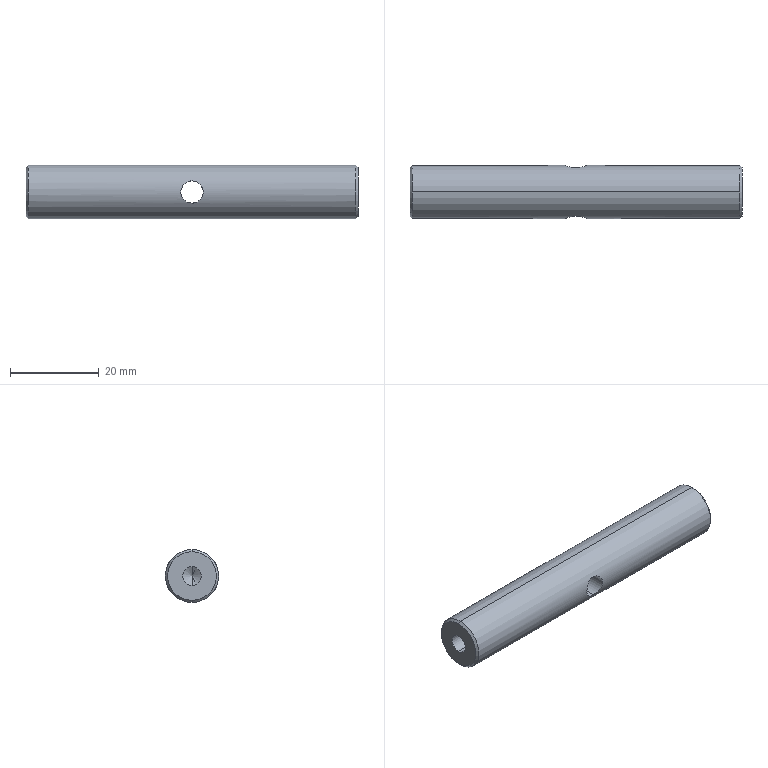Part | SolidWorks | features HoleWzd 2, Chamfer 1, Extrusion 1, ICE 1 | 1 solid | 18 faces | box 75 x 12 x 12 mm | volume 7888 mm3 | cylinder 8 | cone 8 | plane 2 | commonest cylinder face diameters 4.2 x4 5 x2 12 x2
STEP:
#1=CARTESIAN_POINT('',(37.5,-5.454,-2.5));
#2=VERTEX_POINT('',#1);
#3=CARTESIAN_POINT('',(37.5,-5.454,2.5));
#4=VERTEX_POINT('',#3);
#5=CARTESIAN_POINT('',(37.5,-5.454,-2.5));
#6=CARTESIAN_POINT('',(37.335,-5.454,-2.5));
#7=CARTESIAN_POINT('',(37.168,-5.462,-2.483));
#8=CARTESIAN_POINT('',(36.845,-5.491,-2.418));
#9=CARTESIAN_POINT('',(36.688,-5.512,-2.37));
#10=CARTESIAN_POINT('',(36.386,-5.565,-2.244));
#11=CARTESIAN_POINT('',(36.241,-5.596,-2.166));
#12=CARTESIAN_POINT('',(35.972,-5.663,-1.986));
#13=CARTESIAN_POINT('',(35.847,-5.698,-1.882));
#14=CARTESIAN_POINT('',(35.617,-5.769,-1.652));
#15=CARTESIAN_POINT('',(35.515,-5.804,-1.528));
#16=CARTESIAN_POINT('',(35.334,-5.868,-1.259));
#17=CARTESIAN_POINT('',(35.256,-5.898,-1.114));
#18=CARTESIAN_POINT('',(35.13,-5.947,-0.8118));
#19=CARTESIAN_POINT('',(35.082,-5.966,-0.6557));
#20=CARTESIAN_POINT('',(35.017,-5.993,-0.3328));
#21=CARTESIAN_POINT('',(35.,-6.,-0.1652));
#22=CARTESIAN_POINT('',(35.,-6.,0.3293));
#23=CARTESIAN_POINT('',(35.067,-5.971,0.6615));
#24=CARTESIAN_POINT('',(35.256,-5.898,1.114));
#25=CARTESIAN_POINT('',(35.334,-5.868,1.259));
#26=CARTESIAN_POINT('',(35.515,-5.804,1.529));
#27=CARTESIAN_POINT('',(35.618,-5.769,1.653));
#28=CARTESIAN_POINT('',(35.847,-5.698,1.883));
#29=CARTESIAN_POINT('',(35.974,-5.662,1.987));
#30=CARTESIAN_POINT('',(36.242,-5.596,2.166));
#31=CARTESIAN_POINT('',(36.385,-5.565,2.243));
#32=CARTESIAN_POINT('',(36.689,-5.512,2.371));
#33=CARTESIAN_POINT('',(36.845,-5.491,2.418));
#34=CARTESIAN_POINT('',(37.167,-5.462,2.483));
#35=CARTESIAN_POINT('',(37.333,-5.454,2.5));
#36=CARTESIAN_POINT('',(37.5,-5.454,2.5));
#37=B_SPLINE_CURVE_WITH_KNOTS('',3,(#5,#6,#7,#8,#9,#10,#11,#12,#13,#14,#15,#16,#17,#18,#19,#20,#21,#22,#23,#24,#25,#26,#27,#28,#29,#30,#31,#32,#33,#34,#35,#36),.UNSPECIFIED.,.F.,.F.,(4,2,2,2,2,2,2,2,2,2,2,2,2,2,2,4),(0.007907,0.008401,0.008895,0.009388,0.009882,0.01038,0.01087,0.01136,0.01186,0.01284,0.01334,0.01383,0.01433,0.01482,0.01531,0.01581),.UNSPECIFIED.);
#38=EDGE_CURVE('',#2,#4,#37,.T.);
#39=ORIENTED_EDGE('',*,*,#38,.F.);
#40=CARTESIAN_POINT('',(37.5,5.454,-2.5));
#41=VERTEX_POINT('',#40);
#42=CARTESIAN_POINT('',(37.5,-17.,-2.5));
#43=DIRECTION('',(0.,1.,0.));
#44=VECTOR('',#43,1000.);
#45=LINE('',#42,#44);
#46=EDGE_CURVE('',#2,#41,#45,.T.);
#47=ORIENTED_EDGE('',*,*,#46,.T.);
#48=CARTESIAN_POINT('',(37.5,5.454,2.5));
#49=VERTEX_POINT('',#48);
#50=CARTESIAN_POINT('',(37.5,5.454,2.5));
#51=CARTESIAN_POINT('',(37.333,5.454,2.5));
#52=CARTESIAN_POINT('',(37.169,5.462,2.483));
#53=CARTESIAN_POINT('',(36.847,5.491,2.419));
#54=CARTESIAN_POINT('',(36.687,5.513,2.37));
#55=CARTESIAN_POINT('',(36.385,5.565,2.244));
#56=CARTESIAN_POINT('',(36.243,5.596,2.167));
#57=CARTESIAN_POINT('',(35.972,5.663,1.986));
#58=CARTESIAN_POINT('',(35.846,5.699,1.882));
#59=CARTESIAN_POINT('',(35.504,5.804,1.54));
#60=CARTESIAN_POINT('',(35.319,5.873,1.264));
#61=CARTESIAN_POINT('',(35.131,5.947,0.8137));
#62=CARTESIAN_POINT('',(35.081,5.966,0.6541));
#63=CARTESIAN_POINT('',(35.016,5.993,0.3303));
#64=CARTESIAN_POINT('',(35.,6.,0.1667));
#65=CARTESIAN_POINT('',(35.,6.,-0.164));
#66=CARTESIAN_POINT('',(35.017,5.993,-0.3317));
#67=CARTESIAN_POINT('',(35.082,5.966,-0.6542));
#68=CARTESIAN_POINT('',(35.13,5.947,-0.8116));
#69=CARTESIAN_POINT('',(35.257,5.897,-1.116));
#70=CARTESIAN_POINT('',(35.334,5.868,-1.259));
#71=CARTESIAN_POINT('',(35.515,5.804,-1.529));
#72=CARTESIAN_POINT('',(35.62,5.768,-1.656));
#73=CARTESIAN_POINT('',(35.849,5.698,-1.884));
#74=CARTESIAN_POINT('',(35.973,5.663,-1.986));
#75=CARTESIAN_POINT('',(36.243,5.596,-2.167));
#76=CARTESIAN_POINT('',(36.388,5.565,-2.245));
#77=CARTESIAN_POINT('',(36.688,5.512,-2.37));
#78=CARTESIAN_POINT('',(36.844,5.491,-2.418));
#79=CARTESIAN_POINT('',(37.17,5.462,-2.484));
#80=CARTESIAN_POINT('',(37.335,5.454,-2.5));
#81=CARTESIAN_POINT('',(37.5,5.454,-2.5));
#82=B_SPLINE_CURVE_WITH_KNOTS('',3,(#50,#51,#52,#53,#54,#55,#56,#57,#58,#59,#60,#61,#62,#63,#64,#65,#66,#67,#68,#69,#70,#71,#72,#73,#74,#75,#76,#77,#78,#79,#80,#81),.UNSPECIFIED.,.F.,.F.,(4,2,2,2,2,2,2,2,2,2,2,2,2,2,2,4),(0.,0.0004942,0.0009884,0.001483,0.001977,0.002965,0.003459,0.003953,0.004448,0.004942,0.005436,0.00593,0.006424,0.006919,0.007413,0.007907),.UNSPECIFIED.);
#83=EDGE_CURVE('',#49,#41,#82,.T.);
#84=ORIENTED_EDGE('',*,*,#83,.F.);
#85=CARTESIAN_POINT('',(37.5,-17.,2.5));
#86=DIRECTION('',(0.,1.,0.));
#87=VECTOR('',#86,1000.);
#88=LINE('',#85,#87);
#89=EDGE_CURVE('',#4,#49,#88,.T.);
#90=ORIENTED_EDGE('',*,*,#89,.F.);
#91=EDGE_LOOP('',(#39,#47,#84,#90));
#92=FACE_OUTER_BOUND('',#91,.T.);
#93=CARTESIAN_POINT('',(37.5,-17.,0.));
#94=DIRECTION('',(0.,1.,0.));
#95=DIRECTION('',(0.,0.,1.));
#96=AXIS2_PLACEMENT_3D('',#93,#94,#95);
#97=CYLINDRICAL_SURFACE('',#96,2.5);
#98=ADVANCED_FACE('',(#92),#97,.F.);
#99=CARTESIAN_POINT('',(0.,0.,5.5));
#100=VERTEX_POINT('',#99);
#101=CARTESIAN_POINT('',(0.,0.,-5.5));
#102=VERTEX_POINT('',#101);
#103=CARTESIAN_POINT('',(0.,0.,0.));
#104=DIRECTION('',(-1.,0.,0.));
#105=DIRECTION('',(0.,0.,-1.));
#106=AXIS2_PLACEMENT_3D('',#103,#104,#105);
#107=CIRCLE('',#106,5.5);
#108=EDGE_CURVE('',#100,#102,#107,.T.);
#109=ORIENTED_EDGE('',*,*,#108,.F.);
#110=CARTESIAN_POINT('',(0.5,0.,6.));
#111=VERTEX_POINT('',#110);
#112=CARTESIAN_POINT('',(0.5,0.,6.));
#113=DIRECTION('',(0.7071,0.,0.7071));
#114=VECTOR('',#113,1000.);
#115=LINE('',#112,#114);
#116=EDGE_CURVE('',#100,#111,#115,.T.);
#117=ORIENTED_EDGE('',*,*,#116,.T.);
#118=CARTESIAN_POINT('',(0.5,0.,-6.));
#119=VERTEX_POINT('',#118);
#120=CARTESIAN_POINT('',(0.5,0.,0.));
#121=DIRECTION('',(1.,0.,0.));
#122=DIRECTION('',(0.,0.,-1.));
#123=AXIS2_PLACEMENT_3D('',#120,#121,#122);
#124=CIRCLE('',#123,6.);
#125=EDGE_CURVE('',#119,#111,#124,.T.);
#126=ORIENTED_EDGE('',*,*,#125,.F.);
#127=CARTESIAN_POINT('',(0.5,0.,-6.));
#128=DIRECTION('',(0.7071,0.,-0.7071));
#129=VECTOR('',#128,1000.);
#130=LINE('',#127,#129);
#131=EDGE_CURVE('',#102,#119,#130,.T.);
#132=ORIENTED_EDGE('',*,*,#131,.F.);
#133=EDGE_LOOP('',(#109,#117,#126,#132));
#134=FACE_OUTER_BOUND('',#133,.T.);
#135=CARTESIAN_POINT('',(0.5,0.,0.));
#136=DIRECTION('',(1.,0.,0.));
#137=DIRECTION('',(0.,0.,-1.));
#138=AXIS2_PLACEMENT_3D('',#135,#136,#137);
#139=CONICAL_SURFACE('',#138,6.,0.7854);
#140=ADVANCED_FACE('',(#134),#139,.T.);
#141=CARTESIAN_POINT('',(75.,0.,-5.5));
#142=VERTEX_POINT('',#141);
#143=CARTESIAN_POINT('',(75.,0.,5.5));
#144=VERTEX_POINT('',#143);
#145=CARTESIAN_POINT('',(75.,0.,0.));
#146=DIRECTION('',(1.,0.,0.));
#147=DIRECTION('',(0.,0.,-1.));
#148=AXIS2_PLACEMENT_3D('',#145,#146,#147);
#149=CIRCLE('',#148,5.5);
#150=EDGE_CURVE('',#142,#144,#149,.T.);
#151=ORIENTED_EDGE('',*,*,#150,.F.);
#152=CARTESIAN_POINT('',(74.5,0.,-6.));
#153=VERTEX_POINT('',#152);
#154=CARTESIAN_POINT('',(75.,0.,-5.5));
#155=DIRECTION('',(-0.7071,0.,-0.7071));
#156=VECTOR('',#155,1000.);
#157=LINE('',#154,#156);
#158=EDGE_CURVE('',#142,#153,#157,.T.);
#159=ORIENTED_EDGE('',*,*,#158,.T.);
#160=CARTESIAN_POINT('',(74.5,0.,6.));
#161=VERTEX_POINT('',#160);
#162=CARTESIAN_POINT('',(74.5,0.,0.));
#163=DIRECTION('',(-1.,0.,0.));
#164=DIRECTION('',(0.,0.,-1.));
#165=AXIS2_PLACEMENT_3D('',#162,#163,#164);
#166=CIRCLE('',#165,6.);
#167=EDGE_CURVE('',#161,#153,#166,.T.);
#168=ORIENTED_EDGE('',*,*,#167,.F.);
#169=CARTESIAN_POINT('',(75.,0.,5.5));
#170=DIRECTION('',(-0.7071,0.,0.7071));
#171=VECTOR('',#170,1000.);
#172=LINE('',#169,#171);
#173=EDGE_CURVE('',#144,#161,#172,.T.);
#174=ORIENTED_EDGE('',*,*,#173,.F.);
#175=EDGE_LOOP('',(#151,#159,#168,#174));
#176=FACE_OUTER_BOUND('',#175,.T.);
#177=CARTESIAN_POINT('',(75.,0.,0.));
#178=DIRECTION('',(-1.,0.,0.));
#179=DIRECTION('',(0.,0.,1.));
#180=AXIS2_PLACEMENT_3D('',#177,#178,#179);
#181=CONICAL_SURFACE('',#180,5.5,0.7854);
#182=ADVANCED_FACE('',(#176),#181,.T.);
#183=CARTESIAN_POINT('',(12.4,0.,-2.1));
#184=VERTEX_POINT('',#183);
#185=CARTESIAN_POINT('',(12.4,0.,2.1));
#186=VERTEX_POINT('',#185);
#187=CARTESIAN_POINT('',(12.4,0.,0.));
#188=DIRECTION('',(-1.,0.,0.));
#189=DIRECTION('',(0.,0.,1.));
#190=AXIS2_PLACEMENT_3D('',#187,#188,#189);
#191=CIRCLE('',#190,2.1);
#192=EDGE_CURVE('',#184,#186,#191,.T.);
#193=ORIENTED_EDGE('',*,*,#192,.F.);
#194=CARTESIAN_POINT('',(0.,0.,-2.1));
#195=VERTEX_POINT('',#194);
#196=CARTESIAN_POINT('',(0.,0.,-2.1));
#197=DIRECTION('',(-1.,0.,0.));
#198=VECTOR('',#197,1000.);
#199=LINE('',#196,#198);
#200=EDGE_CURVE('',#184,#195,#199,.T.);
#201=ORIENTED_EDGE('',*,*,#200,.T.);
#202=CARTESIAN_POINT('',(0.,0.,2.1));
#203=VERTEX_POINT('',#202);
#204=CARTESIAN_POINT('',(0.,0.,0.));
#205=DIRECTION('',(-1.,0.,0.));
#206=DIRECTION('',(0.,0.,1.));
#207=AXIS2_PLACEMENT_3D('',#204,#205,#206);
#208=CIRCLE('',#207,2.1);
#209=EDGE_CURVE('',#195,#203,#208,.T.);
#210=ORIENTED_EDGE('',*,*,#209,.T.);
#211=CARTESIAN_POINT('',(0.,0.,2.1));
#212=DIRECTION('',(-1.,0.,0.));
#213=VECTOR('',#212,1000.);
#214=LINE('',#211,#213);
#215=EDGE_CURVE('',#186,#203,#214,.T.);
#216=ORIENTED_EDGE('',*,*,#215,.F.);
#217=EDGE_LOOP('',(#193,#201,#210,#216));
#218=FACE_OUTER_BOUND('',#217,.T.);
#219=CARTESIAN_POINT('',(0.,0.,0.));
#220=DIRECTION('',(-1.,0.,0.));
#221=DIRECTION('',(0.,0.,1.));
#222=AXIS2_PLACEMENT_3D('',#219,#220,#221);
#223=CYLINDRICAL_SURFACE('',#222,2.1);
#224=ADVANCED_FACE('',(#218),#223,.F.);
#225=CARTESIAN_POINT('',(13.662,0.,0.));
#226=VERTEX_POINT('',#225);
#227=CARTESIAN_POINT('',(12.4,0.,2.1));
#228=DIRECTION('',(-0.515,0.,0.8572));
#229=VECTOR('',#228,1000.);
#230=LINE('',#227,#229);
#231=EDGE_CURVE('',#226,#186,#230,.T.);
#232=ORIENTED_EDGE('',*,*,#231,.F.);
#233=CARTESIAN_POINT('',(12.4,0.,-2.1));
#234=DIRECTION('',(-0.515,0.,-0.8572));
#235=VECTOR('',#234,1000.);
#236=LINE('',#233,#235);
#237=EDGE_CURVE('',#226,#184,#236,.T.);
#238=ORIENTED_EDGE('',*,*,#237,.T.);
#239=ORIENTED_EDGE('',*,*,#192,.T.);
#240=EDGE_LOOP('',(#232,#238,#239));
#241=FACE_OUTER_BOUND('',#240,.T.);
#242=CARTESIAN_POINT('',(12.4,0.,0.));
#243=DIRECTION('',(-1.,0.,0.));
#244=DIRECTION('',(0.,0.,1.));
#245=AXIS2_PLACEMENT_3D('',#242,#243,#244);
#246=CONICAL_SURFACE('',#245,2.1,1.03);
#247=ADVANCED_FACE('',(#241),#246,.F.);
#248=CARTESIAN_POINT('',(62.6,0.,2.1));
#249=VERTEX_POINT('',#248);
#250=CARTESIAN_POINT('',(62.6,0.,-2.1));
#251=VERTEX_POINT('',#250);
#252=CARTESIAN_POINT('',(62.6,0.,0.));
#253=DIRECTION('',(1.,0.,0.));
#254=DIRECTION('',(0.,0.,-1.));
#255=AXIS2_PLACEMENT_3D('',#252,#253,#254);
#256=CIRCLE('',#255,2.1);
#257=EDGE_CURVE('',#249,#251,#256,.T.);
#258=ORIENTED_EDGE('',*,*,#257,.F.);
#259=CARTESIAN_POINT('',(75.,0.,2.1));
#260=VERTEX_POINT('',#259);
#261=CARTESIAN_POINT('',(75.,0.,2.1));
#262=DIRECTION('',(1.,0.,0.));
#263=VECTOR('',#262,1000.);
#264=LINE('',#261,#263);
#265=EDGE_CURVE('',#249,#260,#264,.T.);
#266=ORIENTED_EDGE('',*,*,#265,.T.);
#267=CARTESIAN_POINT('',(75.,0.,-2.1));
#268=VERTEX_POINT('',#267);
#269=CARTESIAN_POINT('',(75.,0.,0.));
#270=DIRECTION('',(1.,0.,0.));
#271=DIRECTION('',(0.,0.,-1.));
#272=AXIS2_PLACEMENT_3D('',#269,#270,#271);
#273=CIRCLE('',#272,2.1);
#274=EDGE_CURVE('',#260,#268,#273,.T.);
#275=ORIENTED_EDGE('',*,*,#274,.T.);
#276=CARTESIAN_POINT('',(75.,0.,-2.1));
#277=DIRECTION('',(1.,0.,0.));
#278=VECTOR('',#277,1000.);
#279=LINE('',#276,#278);
#280=EDGE_CURVE('',#251,#268,#279,.T.);
#281=ORIENTED_EDGE('',*,*,#280,.F.);
#282=EDGE_LOOP('',(#258,#266,#275,#281));
#283=FACE_OUTER_BOUND('',#282,.T.);
#284=CARTESIAN_POINT('',(75.,0.,0.));
#285=DIRECTION('',(1.,0.,0.));
#286=DIRECTION('',(0.,0.,-1.));
#287=AXIS2_PLACEMENT_3D('',#284,#285,#286);
#288=CYLINDRICAL_SURFACE('',#287,2.1);
#289=ADVANCED_FACE('',(#283),#288,.F.);
#290=CARTESIAN_POINT('',(61.338,0.,0.));
#291=VERTEX_POINT('',#290);
#292=CARTESIAN_POINT('',(62.6,0.,-2.1));
#293=DIRECTION('',(0.515,0.,-0.8572));
#294=VECTOR('',#293,1000.);
#295=LINE('',#292,#294);
#296=EDGE_CURVE('',#291,#251,#295,.T.);
#297=ORIENTED_EDGE('',*,*,#296,.F.);
#298=CARTESIAN_POINT('',(62.6,0.,2.1));
#299=DIRECTION('',(0.515,0.,0.8572));
#300=VECTOR('',#299,1000.);
#301=LINE('',#298,#300);
#302=EDGE_CURVE('',#291,#249,#301,.T.);
#303=ORIENTED_EDGE('',*,*,#302,.T.);
#304=ORIENTED_EDGE('',*,*,#257,.T.);
#305=EDGE_LOOP('',(#297,#303,#304));
#306=FACE_OUTER_BOUND('',#305,.T.);
#307=CARTESIAN_POINT('',(62.6,0.,0.));
#308=DIRECTION('',(1.,0.,0.));
#309=DIRECTION('',(0.,0.,-1.));
#310=AXIS2_PLACEMENT_3D('',#307,#308,#309);
#311=CONICAL_SURFACE('',#310,2.1,1.03);
#312=ADVANCED_FACE('',(#306),#311,.F.);
#313=ORIENTED_EDGE('',*,*,#83,.T.);
#314=CARTESIAN_POINT('',(37.5,5.454,-2.5));
#315=CARTESIAN_POINT('',(37.665,5.454,-2.5));
#316=CARTESIAN_POINT('',(37.832,5.462,-2.483));
#317=CARTESIAN_POINT('',(38.155,5.491,-2.418));
#318=CARTESIAN_POINT('',(38.312,5.512,-2.37));
#319=CARTESIAN_POINT('',(38.614,5.565,-2.244));
#320=CARTESIAN_POINT('',(38.759,5.596,-2.166));
#321=CARTESIAN_POINT('',(39.028,5.663,-1.986));
#322=CARTESIAN_POINT('',(39.153,5.698,-1.882));
#323=CARTESIAN_POINT('',(39.383,5.769,-1.652));
#324=CARTESIAN_POINT('',(39.485,5.804,-1.528));
#325=CARTESIAN_POINT('',(39.666,5.868,-1.259));
#326=CARTESIAN_POINT('',(39.744,5.898,-1.114));
#327=CARTESIAN_POINT('',(39.87,5.947,-0.8118));
#328=CARTESIAN_POINT('',(39.918,5.966,-0.6557));
#329=CARTESIAN_POINT('',(39.983,5.993,-0.3328));
#330=CARTESIAN_POINT('',(40.,6.,-0.1652));
#331=CARTESIAN_POINT('',(40.,6.,0.3293));
#332=CARTESIAN_POINT('',(39.933,5.971,0.6615));
#333=CARTESIAN_POINT('',(39.744,5.898,1.114));
#334=CARTESIAN_POINT('',(39.666,5.868,1.259));
#335=CARTESIAN_POINT('',(39.485,5.804,1.529));
#336=CARTESIAN_POINT('',(39.382,5.769,1.653));
#337=CARTESIAN_POINT('',(39.153,5.698,1.883));
#338=CARTESIAN_POINT('',(39.026,5.662,1.987));
#339=CARTESIAN_POINT('',(38.758,5.596,2.166));
#340=CARTESIAN_POINT('',(38.615,5.565,2.243));
#341=CARTESIAN_POINT('',(38.311,5.512,2.371));
#342=CARTESIAN_POINT('',(38.155,5.491,2.418));
#343=CARTESIAN_POINT('',(37.833,5.462,2.483));
#344=CARTESIAN_POINT('',(37.667,5.454,2.5));
#345=CARTESIAN_POINT('',(37.5,5.454,2.5));
#346=B_SPLINE_CURVE_WITH_KNOTS('',3,(#314,#315,#316,#317,#318,#319,#320,#321,#322,#323,#324,#325,#326,#327,#328,#329,#330,#331,#332,#333,#334,#335,#336,#337,#338,#339,#340,#341,#342,#343,#344,#345),.UNSPECIFIED.,.F.,.F.,(4,2,2,2,2,2,2,2,2,2,2,2,2,2,2,4),(0.007907,0.008401,0.008895,0.009388,0.009882,0.01038,0.01087,0.01136,0.01186,0.01284,0.01334,0.01383,0.01433,0.01482,0.01531,0.01581),.UNSPECIFIED.);
#347=EDGE_CURVE('',#41,#49,#346,.T.);
#348=ORIENTED_EDGE('',*,*,#347,.T.);
#349=EDGE_LOOP('',(#313,#348));
#350=FACE_BOUND('',#349,.T.);
#351=ORIENTED_EDGE('',*,*,#167,.T.);
#352=CARTESIAN_POINT('',(75.,0.,-6.));
#353=DIRECTION('',(-1.,0.,0.));
#354=VECTOR('',#353,1000.);
#355=LINE('',#352,#354);
#356=EDGE_CURVE('',#153,#119,#355,.T.);
#357=ORIENTED_EDGE('',*,*,#356,.T.);
#358=ORIENTED_EDGE('',*,*,#125,.T.);
#359=CARTESIAN_POINT('',(75.,0.,6.));
#360=DIRECTION('',(-1.,0.,0.));
#361=VECTOR('',#360,1000.);
#362=LINE('',#359,#361);
#363=EDGE_CURVE('',#161,#111,#362,.T.);
#364=ORIENTED_EDGE('',*,*,#363,.F.);
#365=EDGE_LOOP('',(#351,#357,#358,#364));
#366=FACE_OUTER_BOUND('',#365,.T.);
#367=CARTESIAN_POINT('',(75.,0.,0.));
#368=DIRECTION('',(-1.,0.,0.));
#369=DIRECTION('',(0.,0.,1.));
#370=AXIS2_PLACEMENT_3D('',#367,#368,#369);
#371=CYLINDRICAL_SURFACE('',#370,6.);
#372=ADVANCED_FACE('',(#350,#366),#371,.T.);
#373=ORIENTED_EDGE('',*,*,#356,.F.);
#374=CARTESIAN_POINT('',(74.5,0.,0.));
#375=DIRECTION('',(-1.,0.,0.));
#376=DIRECTION('',(0.,0.,-1.));
#377=AXIS2_PLACEMENT_3D('',#374,#375,#376);
#378=CIRCLE('',#377,6.);
#379=EDGE_CURVE('',#153,#161,#378,.T.);
#380=ORIENTED_EDGE('',*,*,#379,.T.);
#381=ORIENTED_EDGE('',*,*,#363,.T.);
#382=CARTESIAN_POINT('',(0.5,0.,0.));
#383=DIRECTION('',(1.,0.,0.));
#384=DIRECTION('',(0.,0.,-1.));
#385=AXIS2_PLACEMENT_3D('',#382,#383,#384);
#386=CIRCLE('',#385,6.);
#387=EDGE_CURVE('',#111,#119,#386,.T.);
#388=ORIENTED_EDGE('',*,*,#387,.T.);
#389=EDGE_LOOP('',(#373,#380,#381,#388));
#390=FACE_OUTER_BOUND('',#389,.T.);
#391=CARTESIAN_POINT('',(37.5,-5.454,2.5));
#392=CARTESIAN_POINT('',(37.667,-5.454,2.5));
#393=CARTESIAN_POINT('',(37.831,-5.462,2.483));
#394=CARTESIAN_POINT('',(38.153,-5.491,2.419));
#395=CARTESIAN_POINT('',(38.313,-5.513,2.37));
#396=CARTESIAN_POINT('',(38.615,-5.565,2.244));
#397=CARTESIAN_POINT('',(38.757,-5.596,2.167));
#398=CARTESIAN_POINT('',(39.028,-5.663,1.986));
#399=CARTESIAN_POINT('',(39.154,-5.699,1.882));
#400=CARTESIAN_POINT('',(39.496,-5.804,1.54));
#401=CARTESIAN_POINT('',(39.681,-5.873,1.264));
#402=CARTESIAN_POINT('',(39.869,-5.947,0.8137));
#403=CARTESIAN_POINT('',(39.919,-5.966,0.6541));
#404=CARTESIAN_POINT('',(39.984,-5.993,0.3303));
#405=CARTESIAN_POINT('',(40.,-6.,0.1667));
#406=CARTESIAN_POINT('',(40.,-6.,-0.164));
#407=CARTESIAN_POINT('',(39.983,-5.993,-0.3317));
#408=CARTESIAN_POINT('',(39.918,-5.966,-0.6542));
#409=CARTESIAN_POINT('',(39.87,-5.947,-0.8116));
#410=CARTESIAN_POINT('',(39.743,-5.897,-1.116));
#411=CARTESIAN_POINT('',(39.666,-5.868,-1.259));
#412=CARTESIAN_POINT('',(39.485,-5.804,-1.529));
#413=CARTESIAN_POINT('',(39.38,-5.768,-1.656));
#414=CARTESIAN_POINT('',(39.151,-5.698,-1.884));
#415=CARTESIAN_POINT('',(39.027,-5.663,-1.986));
#416=CARTESIAN_POINT('',(38.757,-5.596,-2.167));
#417=CARTESIAN_POINT('',(38.612,-5.565,-2.245));
#418=CARTESIAN_POINT('',(38.312,-5.512,-2.37));
#419=CARTESIAN_POINT('',(38.156,-5.491,-2.418));
#420=CARTESIAN_POINT('',(37.83,-5.462,-2.484));
#421=CARTESIAN_POINT('',(37.665,-5.454,-2.5));
#422=CARTESIAN_POINT('',(37.5,-5.454,-2.5));
#423=B_SPLINE_CURVE_WITH_KNOTS('',3,(#391,#392,#393,#394,#395,#396,#397,#398,#399,#400,#401,#402,#403,#404,#405,#406,#407,#408,#409,#410,#411,#412,#413,#414,#415,#416,#417,#418,#419,#420,#421,#422),.UNSPECIFIED.,.F.,.F.,(4,2,2,2,2,2,2,2,2,2,2,2,2,2,2,4),(0.,0.0004942,0.0009884,0.001483,0.001977,0.002965,0.003459,0.003953,0.004448,0.004942,0.005436,0.00593,0.006424,0.006919,0.007413,0.007907),.UNSPECIFIED.);
#424=EDGE_CURVE('',#4,#2,#423,.T.);
#425=ORIENTED_EDGE('',*,*,#424,.T.);
#426=ORIENTED_EDGE('',*,*,#38,.T.);
#427=EDGE_LOOP('',(#425,#426));
#428=FACE_BOUND('',#427,.T.);
#429=CARTESIAN_POINT('',(75.,0.,0.));
#430=DIRECTION('',(-1.,0.,0.));
#431=DIRECTION('',(0.,0.,1.));
#432=AXIS2_PLACEMENT_3D('',#429,#430,#431);
#433=CYLINDRICAL_SURFACE('',#432,6.);
#434=ADVANCED_FACE('',(#390,#428),#433,.T.);
#435=CARTESIAN_POINT('',(75.,0.,0.));
#436=DIRECTION('',(1.,0.,0.));
#437=DIRECTION('',(0.,0.,-1.));
#438=AXIS2_PLACEMENT_3D('',#435,#436,#437);
#439=CIRCLE('',#438,5.5);
#440=EDGE_CURVE('',#144,#142,#439,.T.);
#441=ORIENTED_EDGE('',*,*,#440,.T.);
#442=ORIENTED_EDGE('',*,*,#150,.T.);
#443=EDGE_LOOP('',(#441,#442));
#444=FACE_OUTER_BOUND('',#443,.T.);
#445=CARTESIAN_POINT('',(75.,0.,0.));
#446=DIRECTION('',(1.,0.,0.));
#447=DIRECTION('',(0.,0.,-1.));
#448=AXIS2_PLACEMENT_3D('',#445,#446,#447);
#449=CIRCLE('',#448,2.1);
#450=EDGE_CURVE('',#268,#260,#449,.T.);
#451=ORIENTED_EDGE('',*,*,#450,.F.);
#452=ORIENTED_EDGE('',*,*,#274,.F.);
#453=EDGE_LOOP('',(#451,#452));
#454=FACE_BOUND('',#453,.T.);
#455=CARTESIAN_POINT('',(75.,0.,0.));
#456=DIRECTION('',(1.,0.,0.));
#457=DIRECTION('',(0.,0.,-1.));
#458=AXIS2_PLACEMENT_3D('',#455,#456,#457);
#459=PLANE('',#458);
#460=ADVANCED_FACE('',(#444,#454),#459,.T.);
#461=CARTESIAN_POINT('',(0.,0.,0.));
#462=DIRECTION('',(-1.,0.,0.));
#463=DIRECTION('',(0.,0.,-1.));
#464=AXIS2_PLACEMENT_3D('',#461,#462,#463);
#465=CIRCLE('',#464,5.5);
#466=EDGE_CURVE('',#102,#100,#465,.T.);
#467=ORIENTED_EDGE('',*,*,#466,.T.);
#468=ORIENTED_EDGE('',*,*,#108,.T.);
#469=EDGE_LOOP('',(#467,#468));
#470=FACE_OUTER_BOUND('',#469,.T.);
#471=CARTESIAN_POINT('',(0.,0.,0.));
#472=DIRECTION('',(-1.,0.,0.));
#473=DIRECTION('',(0.,0.,1.));
#474=AXIS2_PLACEMENT_3D('',#471,#472,#473);
#475=CIRCLE('',#474,2.1);
#476=EDGE_CURVE('',#203,#195,#475,.T.);
#477=ORIENTED_EDGE('',*,*,#476,.F.);
#478=ORIENTED_EDGE('',*,*,#209,.F.);
#479=EDGE_LOOP('',(#477,#478));
#480=FACE_BOUND('',#479,.T.);
#481=CARTESIAN_POINT('',(0.,0.,0.));
#482=DIRECTION('',(1.,0.,0.));
#483=DIRECTION('',(0.,0.,-1.));
#484=AXIS2_PLACEMENT_3D('',#481,#482,#483);
#485=PLANE('',#484);
#486=ADVANCED_FACE('',(#470,#480),#485,.F.);
#487=ORIENTED_EDGE('',*,*,#302,.F.);
#488=ORIENTED_EDGE('',*,*,#296,.T.);
#489=CARTESIAN_POINT('',(62.6,0.,0.));
#490=DIRECTION('',(1.,0.,0.));
#491=DIRECTION('',(0.,0.,-1.));
#492=AXIS2_PLACEMENT_3D('',#489,#490,#491);
#493=CIRCLE('',#492,2.1);
#494=EDGE_CURVE('',#251,#249,#493,.T.);
#495=ORIENTED_EDGE('',*,*,#494,.T.);
#496=EDGE_LOOP('',(#487,#488,#495));
#497=FACE_OUTER_BOUND('',#496,.T.);
#498=CARTESIAN_POINT('',(62.6,0.,0.));
#499=DIRECTION('',(1.,0.,0.));
#500=DIRECTION('',(0.,0.,-1.));
#501=AXIS2_PLACEMENT_3D('',#498,#499,#500);
#502=CONICAL_SURFACE('',#501,2.1,1.03);
#503=ADVANCED_FACE('',(#497),#502,.F.);
#504=ORIENTED_EDGE('',*,*,#265,.F.);
#505=ORIENTED_EDGE('',*,*,#494,.F.);
#506=ORIENTED_EDGE('',*,*,#280,.T.);
#507=ORIENTED_EDGE('',*,*,#450,.T.);
#508=EDGE_LOOP('',(#504,#505,#506,#507));
#509=FACE_OUTER_BOUND('',#508,.T.);
#510=CARTESIAN_POINT('',(75.,0.,0.));
#511=DIRECTION('',(1.,0.,0.));
#512=DIRECTION('',(0.,0.,-1.));
#513=AXIS2_PLACEMENT_3D('',#510,#511,#512);
#514=CYLINDRICAL_SURFACE('',#513,2.1);
#515=ADVANCED_FACE('',(#509),#514,.F.);
#516=ORIENTED_EDGE('',*,*,#237,.F.);
#517=ORIENTED_EDGE('',*,*,#231,.T.);
#518=CARTESIAN_POINT('',(12.4,0.,0.));
#519=DIRECTION('',(-1.,0.,0.));
#520=DIRECTION('',(0.,0.,1.));
#521=AXIS2_PLACEMENT_3D('',#518,#519,#520);
#522=CIRCLE('',#521,2.1);
#523=EDGE_CURVE('',#186,#184,#522,.T.);
#524=ORIENTED_EDGE('',*,*,#523,.T.);
#525=EDGE_LOOP('',(#516,#517,#524));
#526=FACE_OUTER_BOUND('',#525,.T.);
#527=CARTESIAN_POINT('',(12.4,0.,0.));
#528=DIRECTION('',(-1.,0.,0.));
#529=DIRECTION('',(0.,0.,1.));
#530=AXIS2_PLACEMENT_3D('',#527,#528,#529);
#531=CONICAL_SURFACE('',#530,2.1,1.03);
#532=ADVANCED_FACE('',(#526),#531,.F.);
#533=ORIENTED_EDGE('',*,*,#200,.F.);
#534=ORIENTED_EDGE('',*,*,#523,.F.);
#535=ORIENTED_EDGE('',*,*,#215,.T.);
#536=ORIENTED_EDGE('',*,*,#476,.T.);
#537=EDGE_LOOP('',(#533,#534,#535,#536));
#538=FACE_OUTER_BOUND('',#537,.T.);
#539=CARTESIAN_POINT('',(0.,0.,0.));
#540=DIRECTION('',(-1.,0.,0.));
#541=DIRECTION('',(0.,0.,1.));
#542=AXIS2_PLACEMENT_3D('',#539,#540,#541);
#543=CYLINDRICAL_SURFACE('',#542,2.1);
#544=ADVANCED_FACE('',(#538),#543,.F.);
#545=ORIENTED_EDGE('',*,*,#158,.F.);
#546=ORIENTED_EDGE('',*,*,#440,.F.);
#547=ORIENTED_EDGE('',*,*,#173,.T.);
#548=ORIENTED_EDGE('',*,*,#379,.F.);
#549=EDGE_LOOP('',(#545,#546,#547,#548));
#550=FACE_OUTER_BOUND('',#549,.T.);
#551=CARTESIAN_POINT('',(75.,0.,0.));
#552=DIRECTION('',(-1.,0.,0.));
#553=DIRECTION('',(0.,0.,1.));
#554=AXIS2_PLACEMENT_3D('',#551,#552,#553);
#555=CONICAL_SURFACE('',#554,5.5,0.7854);
#556=ADVANCED_FACE('',(#550),#555,.T.);
#557=ORIENTED_EDGE('',*,*,#116,.F.);
#558=ORIENTED_EDGE('',*,*,#466,.F.);
#559=ORIENTED_EDGE('',*,*,#131,.T.);
#560=ORIENTED_EDGE('',*,*,#387,.F.);
#561=EDGE_LOOP('',(#557,#558,#559,#560));
#562=FACE_OUTER_BOUND('',#561,.T.);
#563=CARTESIAN_POINT('',(0.5,0.,0.));
#564=DIRECTION('',(1.,0.,0.));
#565=DIRECTION('',(0.,0.,-1.));
#566=AXIS2_PLACEMENT_3D('',#563,#564,#565);
#567=CONICAL_SURFACE('',#566,6.,0.7854);
#568=ADVANCED_FACE('',(#562),#567,.T.);
#569=ORIENTED_EDGE('',*,*,#46,.F.);
#570=ORIENTED_EDGE('',*,*,#424,.F.);
#571=ORIENTED_EDGE('',*,*,#89,.T.);
#572=ORIENTED_EDGE('',*,*,#347,.F.);
#573=EDGE_LOOP('',(#569,#570,#571,#572));
#574=FACE_OUTER_BOUND('',#573,.T.);
#575=CARTESIAN_POINT('',(37.5,-17.,0.));
#576=DIRECTION('',(0.,1.,0.));
#577=DIRECTION('',(0.,0.,1.));
#578=AXIS2_PLACEMENT_3D('',#575,#576,#577);
#579=CYLINDRICAL_SURFACE('',#578,2.5);
#580=ADVANCED_FACE('',(#574),#579,.F.);
#581=CLOSED_SHELL('',(#98,#140,#182,#224,#247,#289,#312,#372,#434,#460,#486,#503,#515,#532,#544,#556,#568,#580));
#582=MANIFOLD_SOLID_BREP('',#581);
#583=CARTESIAN_POINT('',(0.,0.,0.));
#584=DIRECTION('',(0.,0.,1.));
#585=DIRECTION('',(1.,0.,0.));
#586=AXIS2_PLACEMENT_3D('',#583,#584,#585);
#587=(LENGTH_UNIT()NAMED_UNIT(*)SI_UNIT(.MILLI.,.METRE.));
#588=UNCERTAINTY_MEASURE_WITH_UNIT(LENGTH_MEASURE(0.00001),#587,'','');
#589=(NAMED_UNIT(*)PLANE_ANGLE_UNIT()SI_UNIT($,.RADIAN.));
#590=(NAMED_UNIT(*)SI_UNIT($,.STERADIAN.)SOLID_ANGLE_UNIT());
#591=(GEOMETRIC_REPRESENTATION_CONTEXT(3)GLOBAL_UNCERTAINTY_ASSIGNED_CONTEXT((#588))GLOBAL_UNIT_ASSIGNED_CONTEXT((#587,#589,#590))REPRESENTATION_CONTEXT('',''));
#592=ADVANCED_BREP_SHAPE_REPRESENTATION('',(#582,#586),#591);